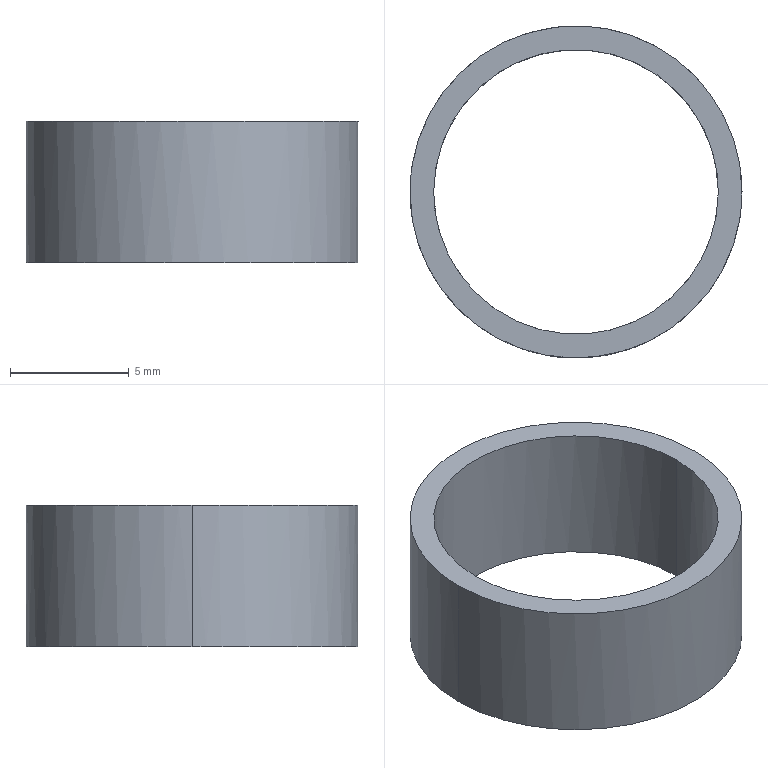Part | SolidWorks | features BaseBody 1 | 1 solid | 6 faces | box 14 x 14 x 5.984 mm | volume 244.304 mm3 | cylinder 4 | plane 2 | commonest cylinder face diameters 12 x2 14 x2
STEP:
#1=CARTESIAN_POINT('',(412.269,212.516,20.485));
#2=VERTEX_POINT('',#1);
#3=CARTESIAN_POINT('',(412.269,212.495,20.485));
#4=VERTEX_POINT('',#3);
#5=CARTESIAN_POINT('',(418.269,212.516,20.485));
#6=DIRECTION('',(0.,0.,1.));
#7=DIRECTION('',(-1.,0.,0.));
#8=AXIS2_PLACEMENT_3D('',#5,#6,#7);
#9=CIRCLE('',#8,6.);
#10=EDGE_CURVE('',#2,#4,#9,.T.);
#11=ORIENTED_EDGE('',*,*,#10,.F.);
#12=CARTESIAN_POINT('',(412.269,212.516,26.469));
#13=VERTEX_POINT('',#12);
#14=CARTESIAN_POINT('',(412.269,212.516,18.477));
#15=DIRECTION('',(0.,0.,1.));
#16=VECTOR('',#15,1000.);
#17=LINE('',#14,#16);
#18=EDGE_CURVE('',#2,#13,#17,.T.);
#19=ORIENTED_EDGE('',*,*,#18,.T.);
#20=CARTESIAN_POINT('',(412.269,212.495,26.469));
#21=VERTEX_POINT('',#20);
#22=CARTESIAN_POINT('',(418.269,212.516,26.469));
#23=DIRECTION('',(0.,0.,-1.));
#24=DIRECTION('',(-1.,-0.003633,0.));
#25=AXIS2_PLACEMENT_3D('',#22,#23,#24);
#26=CIRCLE('',#25,6.);
#27=EDGE_CURVE('',#21,#13,#26,.T.);
#28=ORIENTED_EDGE('',*,*,#27,.F.);
#29=CARTESIAN_POINT('',(424.269,212.516,26.467));
#30=VERTEX_POINT('',#29);
#31=CARTESIAN_POINT('',(424.269,212.516,26.467));
#32=CARTESIAN_POINT('',(424.269,200.56,26.467));
#33=CARTESIAN_POINT('',(412.312,200.538,26.469));
#34=CARTESIAN_POINT('',(412.269,212.495,26.469));
#35=(BOUNDED_CURVE()B_SPLINE_CURVE(3,(#31,#32,#33,#34),.UNSPECIFIED.,.F.,.F.)B_SPLINE_CURVE_WITH_KNOTS((4,4),(3.145,6.283),.UNSPECIFIED.)CURVE()GEOMETRIC_REPRESENTATION_ITEM()RATIONAL_B_SPLINE_CURVE((1.,0.3345,0.3345,1.))REPRESENTATION_ITEM(''));
#36=EDGE_CURVE('',#30,#21,#35,.T.);
#37=ORIENTED_EDGE('',*,*,#36,.F.);
#38=CARTESIAN_POINT('',(424.269,212.516,20.487));
#39=VERTEX_POINT('',#38);
#40=CARTESIAN_POINT('',(424.269,212.516,18.477));
#41=DIRECTION('',(0.,0.,1.));
#42=VECTOR('',#41,1000.);
#43=LINE('',#40,#42);
#44=EDGE_CURVE('',#39,#30,#43,.T.);
#45=ORIENTED_EDGE('',*,*,#44,.F.);
#46=CARTESIAN_POINT('',(412.269,212.495,20.485));
#47=CARTESIAN_POINT('',(412.312,200.538,20.485));
#48=CARTESIAN_POINT('',(424.269,200.56,20.486));
#49=CARTESIAN_POINT('',(424.269,212.516,20.487));
#50=(BOUNDED_CURVE()B_SPLINE_CURVE(3,(#46,#47,#48,#49),.UNSPECIFIED.,.F.,.F.)B_SPLINE_CURVE_WITH_KNOTS((4,4),(3.142,6.28),.UNSPECIFIED.)CURVE()GEOMETRIC_REPRESENTATION_ITEM()RATIONAL_B_SPLINE_CURVE((1.,0.3345,0.3345,1.))REPRESENTATION_ITEM(''));
#51=EDGE_CURVE('',#4,#39,#50,.T.);
#52=ORIENTED_EDGE('',*,*,#51,.F.);
#53=EDGE_LOOP('',(#11,#19,#28,#37,#45,#52));
#54=FACE_OUTER_BOUND('',#53,.T.);
#55=CARTESIAN_POINT('',(418.269,212.516,18.477));
#56=DIRECTION('',(0.,0.,1.));
#57=DIRECTION('',(1.,0.,0.));
#58=AXIS2_PLACEMENT_3D('',#55,#56,#57);
#59=CYLINDRICAL_SURFACE('',#58,6.);
#60=ADVANCED_FACE('',(#54),#59,.F.);
#61=CARTESIAN_POINT('',(411.269,212.516,20.484));
#62=VERTEX_POINT('',#61);
#63=CARTESIAN_POINT('',(425.268,212.542,20.487));
#64=VERTEX_POINT('',#63);
#65=CARTESIAN_POINT('',(411.269,212.516,20.484));
#66=CARTESIAN_POINT('',(411.269,226.466,20.484));
#67=CARTESIAN_POINT('',(425.218,226.491,20.487));
#68=CARTESIAN_POINT('',(425.268,212.542,20.487));
#69=(BOUNDED_CURVE()B_SPLINE_CURVE(3,(#65,#66,#67,#68),.UNSPECIFIED.,.F.,.F.)B_SPLINE_CURVE_WITH_KNOTS((4,4),(3.145,6.283),.UNSPECIFIED.)CURVE()GEOMETRIC_REPRESENTATION_ITEM()RATIONAL_B_SPLINE_CURVE((1.,0.3345,0.3345,1.))REPRESENTATION_ITEM(''));
#70=EDGE_CURVE('',#62,#64,#69,.T.);
#71=ORIENTED_EDGE('',*,*,#70,.F.);
#72=CARTESIAN_POINT('',(411.269,212.516,26.469));
#73=VERTEX_POINT('',#72);
#74=CARTESIAN_POINT('',(411.269,212.516,18.477));
#75=DIRECTION('',(0.,0.,1.));
#76=VECTOR('',#75,1000.);
#77=LINE('',#74,#76);
#78=EDGE_CURVE('',#62,#73,#77,.T.);
#79=ORIENTED_EDGE('',*,*,#78,.T.);
#80=CARTESIAN_POINT('',(425.268,212.542,26.467));
#81=VERTEX_POINT('',#80);
#82=CARTESIAN_POINT('',(425.268,212.542,26.467));
#83=CARTESIAN_POINT('',(425.218,226.491,26.467));
#84=CARTESIAN_POINT('',(411.269,226.466,26.469));
#85=CARTESIAN_POINT('',(411.269,212.516,26.469));
#86=(BOUNDED_CURVE()B_SPLINE_CURVE(3,(#82,#83,#84,#85),.UNSPECIFIED.,.F.,.F.)B_SPLINE_CURVE_WITH_KNOTS((4,4),(3.142,6.28),.UNSPECIFIED.)CURVE()GEOMETRIC_REPRESENTATION_ITEM()RATIONAL_B_SPLINE_CURVE((1.,0.3345,0.3345,1.))REPRESENTATION_ITEM(''));
#87=EDGE_CURVE('',#81,#73,#86,.T.);
#88=ORIENTED_EDGE('',*,*,#87,.F.);
#89=CARTESIAN_POINT('',(425.269,212.516,26.467));
#90=VERTEX_POINT('',#89);
#91=CARTESIAN_POINT('',(418.269,212.516,26.467));
#92=DIRECTION('',(0.,0.,-1.));
#93=DIRECTION('',(1.,0.003633,0.));
#94=AXIS2_PLACEMENT_3D('',#91,#92,#93);
#95=CIRCLE('',#94,7.);
#96=EDGE_CURVE('',#81,#90,#95,.T.);
#97=ORIENTED_EDGE('',*,*,#96,.T.);
#98=CARTESIAN_POINT('',(425.269,212.516,20.487));
#99=VERTEX_POINT('',#98);
#100=CARTESIAN_POINT('',(425.269,212.516,18.477));
#101=DIRECTION('',(0.,0.,1.));
#102=VECTOR('',#101,1000.);
#103=LINE('',#100,#102);
#104=EDGE_CURVE('',#99,#90,#103,.T.);
#105=ORIENTED_EDGE('',*,*,#104,.F.);
#106=CARTESIAN_POINT('',(418.269,212.516,20.487));
#107=DIRECTION('',(0.,0.,1.));
#108=DIRECTION('',(1.,0.,0.));
#109=AXIS2_PLACEMENT_3D('',#106,#107,#108);
#110=CIRCLE('',#109,7.);
#111=EDGE_CURVE('',#99,#64,#110,.T.);
#112=ORIENTED_EDGE('',*,*,#111,.T.);
#113=EDGE_LOOP('',(#71,#79,#88,#97,#105,#112));
#114=FACE_OUTER_BOUND('',#113,.T.);
#115=CARTESIAN_POINT('',(418.269,212.516,18.477));
#116=DIRECTION('',(0.,0.,1.));
#117=DIRECTION('',(1.,0.,0.));
#118=AXIS2_PLACEMENT_3D('',#115,#116,#117);
#119=CYLINDRICAL_SURFACE('',#118,7.);
#120=ADVANCED_FACE('',(#114),#119,.T.);
#121=ORIENTED_EDGE('',*,*,#78,.F.);
#122=CARTESIAN_POINT('',(411.269,212.491,20.484));
#123=VERTEX_POINT('',#122);
#124=CARTESIAN_POINT('',(418.269,212.516,20.484));
#125=DIRECTION('',(0.,0.,1.));
#126=DIRECTION('',(-1.,0.,0.));
#127=AXIS2_PLACEMENT_3D('',#124,#125,#126);
#128=CIRCLE('',#127,7.);
#129=EDGE_CURVE('',#62,#123,#128,.T.);
#130=ORIENTED_EDGE('',*,*,#129,.T.);
#131=CARTESIAN_POINT('',(425.269,212.516,20.487));
#132=CARTESIAN_POINT('',(425.269,198.567,20.487));
#133=CARTESIAN_POINT('',(411.319,198.542,20.484));
#134=CARTESIAN_POINT('',(411.269,212.491,20.484));
#135=(BOUNDED_CURVE()B_SPLINE_CURVE(3,(#131,#132,#133,#134),.UNSPECIFIED.,.F.,.F.)B_SPLINE_CURVE_WITH_KNOTS((4,4),(0.003633,3.142),.UNSPECIFIED.)CURVE()GEOMETRIC_REPRESENTATION_ITEM()RATIONAL_B_SPLINE_CURVE((1.,0.3345,0.3345,1.))REPRESENTATION_ITEM(''));
#136=EDGE_CURVE('',#99,#123,#135,.T.);
#137=ORIENTED_EDGE('',*,*,#136,.F.);
#138=ORIENTED_EDGE('',*,*,#104,.T.);
#139=CARTESIAN_POINT('',(411.269,212.491,26.469));
#140=VERTEX_POINT('',#139);
#141=CARTESIAN_POINT('',(411.269,212.491,26.469));
#142=CARTESIAN_POINT('',(411.319,198.542,26.469));
#143=CARTESIAN_POINT('',(425.269,198.567,26.467));
#144=CARTESIAN_POINT('',(425.269,212.516,26.467));
#145=(BOUNDED_CURVE()B_SPLINE_CURVE(3,(#141,#142,#143,#144),.UNSPECIFIED.,.F.,.F.)B_SPLINE_CURVE_WITH_KNOTS((4,4),(0.,3.138),.UNSPECIFIED.)CURVE()GEOMETRIC_REPRESENTATION_ITEM()RATIONAL_B_SPLINE_CURVE((1.,0.3345,0.3345,1.))REPRESENTATION_ITEM(''));
#146=EDGE_CURVE('',#140,#90,#145,.T.);
#147=ORIENTED_EDGE('',*,*,#146,.F.);
#148=CARTESIAN_POINT('',(418.269,212.516,26.469));
#149=DIRECTION('',(0.,0.,-1.));
#150=DIRECTION('',(-1.,-0.003633,0.));
#151=AXIS2_PLACEMENT_3D('',#148,#149,#150);
#152=CIRCLE('',#151,7.);
#153=EDGE_CURVE('',#140,#73,#152,.T.);
#154=ORIENTED_EDGE('',*,*,#153,.T.);
#155=EDGE_LOOP('',(#121,#130,#137,#138,#147,#154));
#156=FACE_OUTER_BOUND('',#155,.T.);
#157=CARTESIAN_POINT('',(418.269,212.516,18.477));
#158=DIRECTION('',(0.,0.,1.));
#159=DIRECTION('',(1.,0.,0.));
#160=AXIS2_PLACEMENT_3D('',#157,#158,#159);
#161=CYLINDRICAL_SURFACE('',#160,7.);
#162=ADVANCED_FACE('',(#156),#161,.T.);
#163=CARTESIAN_POINT('',(424.268,212.538,26.467));
#164=VERTEX_POINT('',#163);
#165=CARTESIAN_POINT('',(412.269,212.516,26.469));
#166=CARTESIAN_POINT('',(412.269,224.473,26.469));
#167=CARTESIAN_POINT('',(424.225,224.495,26.467));
#168=CARTESIAN_POINT('',(424.268,212.538,26.467));
#169=(BOUNDED_CURVE()B_SPLINE_CURVE(3,(#165,#166,#167,#168),.UNSPECIFIED.,.F.,.F.)B_SPLINE_CURVE_WITH_KNOTS((4,4),(0.003633,3.142),.UNSPECIFIED.)CURVE()GEOMETRIC_REPRESENTATION_ITEM()RATIONAL_B_SPLINE_CURVE((1.,0.3345,0.3345,1.))REPRESENTATION_ITEM(''));
#170=EDGE_CURVE('',#13,#164,#169,.T.);
#171=ORIENTED_EDGE('',*,*,#170,.T.);
#172=CARTESIAN_POINT('',(418.269,212.516,26.467));
#173=DIRECTION('',(0.,0.,-1.));
#174=DIRECTION('',(1.,0.003633,0.));
#175=AXIS2_PLACEMENT_3D('',#172,#173,#174);
#176=CIRCLE('',#175,6.);
#177=EDGE_CURVE('',#164,#30,#176,.T.);
#178=ORIENTED_EDGE('',*,*,#177,.T.);
#179=ORIENTED_EDGE('',*,*,#36,.T.);
#180=ORIENTED_EDGE('',*,*,#27,.T.);
#181=EDGE_LOOP('',(#171,#178,#179,#180));
#182=FACE_BOUND('',#181,.T.);
#183=ORIENTED_EDGE('',*,*,#96,.F.);
#184=ORIENTED_EDGE('',*,*,#87,.T.);
#185=ORIENTED_EDGE('',*,*,#153,.F.);
#186=ORIENTED_EDGE('',*,*,#146,.T.);
#187=EDGE_LOOP('',(#183,#184,#185,#186));
#188=FACE_OUTER_BOUND('',#187,.T.);
#189=CARTESIAN_POINT('',(424.768,212.54,26.467));
#190=DIRECTION('',(0.000154,0.000000559,1.));
#191=DIRECTION('',(0.003633,-1.,0.));
#192=AXIS2_PLACEMENT_3D('',#189,#190,#191);
#193=PLANE('',#192);
#194=ADVANCED_FACE('',(#182,#188),#193,.T.);
#195=ORIENTED_EDGE('',*,*,#18,.F.);
#196=CARTESIAN_POINT('',(424.268,212.538,20.486));
#197=VERTEX_POINT('',#196);
#198=CARTESIAN_POINT('',(424.268,212.538,20.486));
#199=CARTESIAN_POINT('',(424.225,224.495,20.486));
#200=CARTESIAN_POINT('',(412.269,224.473,20.485));
#201=CARTESIAN_POINT('',(412.269,212.516,20.485));
#202=(BOUNDED_CURVE()B_SPLINE_CURVE(3,(#198,#199,#200,#201),.UNSPECIFIED.,.F.,.F.)B_SPLINE_CURVE_WITH_KNOTS((4,4),(0.,3.138),.UNSPECIFIED.)CURVE()GEOMETRIC_REPRESENTATION_ITEM()RATIONAL_B_SPLINE_CURVE((1.,0.3345,0.3345,1.))REPRESENTATION_ITEM(''));
#203=EDGE_CURVE('',#197,#2,#202,.T.);
#204=ORIENTED_EDGE('',*,*,#203,.F.);
#205=CARTESIAN_POINT('',(418.269,212.516,20.486));
#206=DIRECTION('',(0.,0.,1.));
#207=DIRECTION('',(1.,0.,0.));
#208=AXIS2_PLACEMENT_3D('',#205,#206,#207);
#209=CIRCLE('',#208,6.);
#210=EDGE_CURVE('',#39,#197,#209,.T.);
#211=ORIENTED_EDGE('',*,*,#210,.F.);
#212=ORIENTED_EDGE('',*,*,#44,.T.);
#213=ORIENTED_EDGE('',*,*,#177,.F.);
#214=ORIENTED_EDGE('',*,*,#170,.F.);
#215=EDGE_LOOP('',(#195,#204,#211,#212,#213,#214));
#216=FACE_OUTER_BOUND('',#215,.T.);
#217=CARTESIAN_POINT('',(418.269,212.516,18.477));
#218=DIRECTION('',(0.,0.,1.));
#219=DIRECTION('',(1.,0.,0.));
#220=AXIS2_PLACEMENT_3D('',#217,#218,#219);
#221=CYLINDRICAL_SURFACE('',#220,6.);
#222=ADVANCED_FACE('',(#216),#221,.F.);
#223=ORIENTED_EDGE('',*,*,#10,.T.);
#224=ORIENTED_EDGE('',*,*,#51,.T.);
#225=ORIENTED_EDGE('',*,*,#210,.T.);
#226=ORIENTED_EDGE('',*,*,#203,.T.);
#227=EDGE_LOOP('',(#223,#224,#225,#226));
#228=FACE_BOUND('',#227,.T.);
#229=ORIENTED_EDGE('',*,*,#136,.T.);
#230=ORIENTED_EDGE('',*,*,#129,.F.);
#231=ORIENTED_EDGE('',*,*,#70,.T.);
#232=ORIENTED_EDGE('',*,*,#111,.F.);
#233=EDGE_LOOP('',(#229,#230,#231,#232));
#234=FACE_OUTER_BOUND('',#233,.T.);
#235=CARTESIAN_POINT('',(411.769,212.493,20.485));
#236=DIRECTION('',(-0.000154,-0.000000559,1.));
#237=DIRECTION('',(-0.003633,1.,0.));
#238=AXIS2_PLACEMENT_3D('',#235,#236,#237);
#239=PLANE('',#238);
#240=ADVANCED_FACE('',(#228,#234),#239,.F.);
#241=CLOSED_SHELL('',(#60,#120,#162,#194,#222,#240));
#242=MANIFOLD_SOLID_BREP('',#241);
#243=CARTESIAN_POINT('',(0.,0.,0.));
#244=DIRECTION('',(0.,0.,1.));
#245=DIRECTION('',(1.,0.,0.));
#246=AXIS2_PLACEMENT_3D('',#243,#244,#245);
#247=(LENGTH_UNIT()NAMED_UNIT(*)SI_UNIT(.MILLI.,.METRE.));
#248=UNCERTAINTY_MEASURE_WITH_UNIT(LENGTH_MEASURE(0.00001),#247,'','');
#249=(NAMED_UNIT(*)PLANE_ANGLE_UNIT()SI_UNIT($,.RADIAN.));
#250=(NAMED_UNIT(*)SI_UNIT($,.STERADIAN.)SOLID_ANGLE_UNIT());
#251=(GEOMETRIC_REPRESENTATION_CONTEXT(3)GLOBAL_UNCERTAINTY_ASSIGNED_CONTEXT((#248))GLOBAL_UNIT_ASSIGNED_CONTEXT((#247,#249,#250))REPRESENTATION_CONTEXT('',''));
#252=ADVANCED_BREP_SHAPE_REPRESENTATION('',(#242,#246),#251);